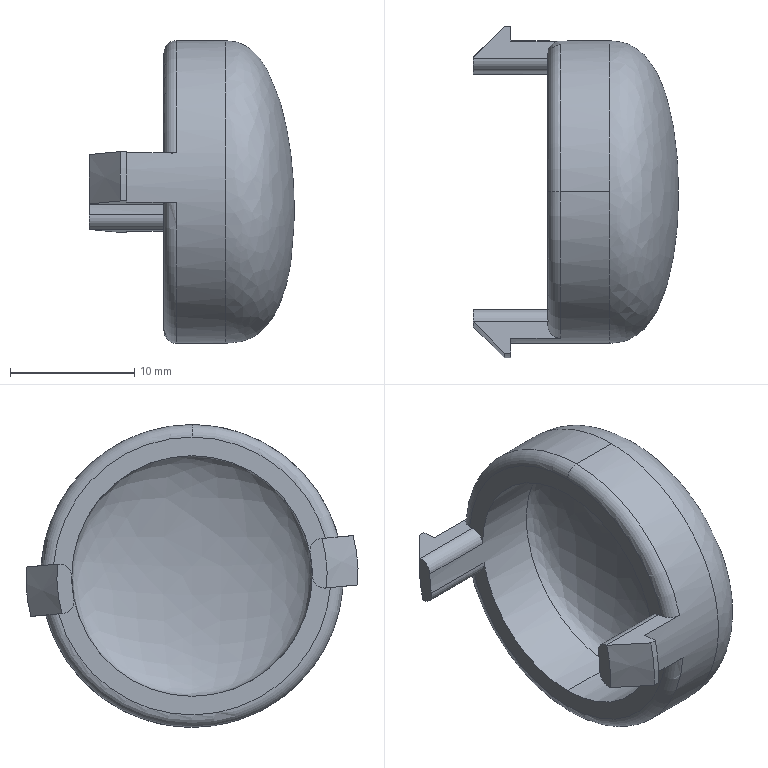Part | SolidWorks | features BaseBody 1 | 1 solid | 28 faces | box 16.535 x 26.8 x 24.4 mm | volume 2199 mm3 | cylinder 11 | plane 10 | torus 3 | spline 2 | cone 2 | commonest cylinder face diameters 2 x5 19.4 x2 24.4 x2 26.8 x2